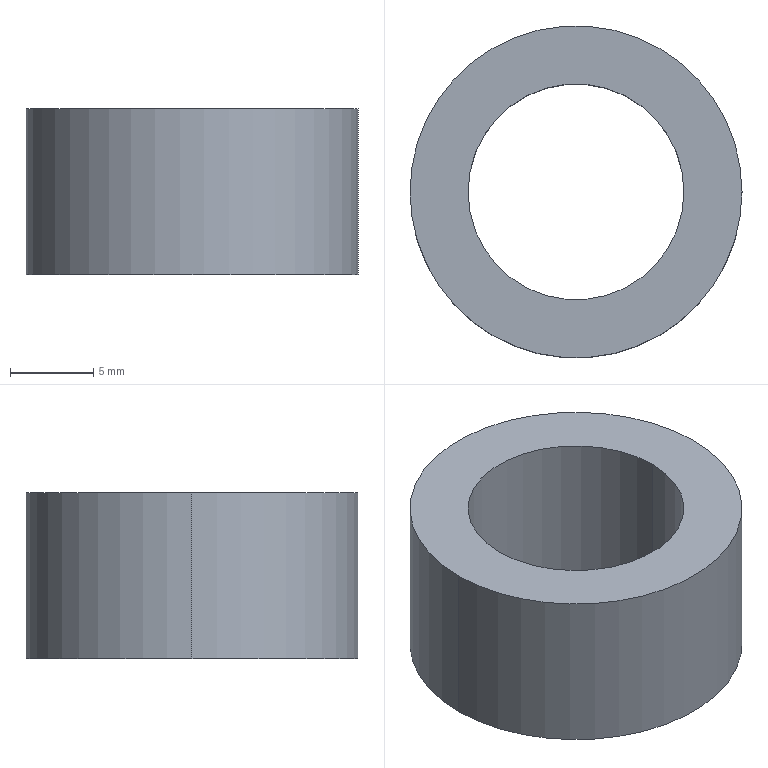Part | SolidWorks | features Cut 1, Extrusion 1 | 1 solid | 6 faces | box 20 x 20 x 10 mm | volume 1814 mm3 | cylinder 4 | plane 2 | commonest cylinder face diameters 13 x2 20 x2
STEP:
#1=CARTESIAN_POINT('',(-6.5,0.,0.));
#2=VERTEX_POINT('',#1);
#3=CARTESIAN_POINT('',(6.5,0.,0.));
#4=VERTEX_POINT('',#3);
#5=CARTESIAN_POINT('',(0.,0.,0.));
#6=DIRECTION('',(0.,0.,1.));
#7=DIRECTION('',(1.,0.,0.));
#8=AXIS2_PLACEMENT_3D('',#5,#6,#7);
#9=CIRCLE('',#8,6.5);
#10=EDGE_CURVE('',#2,#4,#9,.T.);
#11=ORIENTED_EDGE('',*,*,#10,.F.);
#12=CARTESIAN_POINT('',(-6.5,0.,10.));
#13=VERTEX_POINT('',#12);
#14=CARTESIAN_POINT('',(-6.5,0.,0.));
#15=DIRECTION('',(0.,0.,1.));
#16=VECTOR('',#15,1000.);
#17=LINE('',#14,#16);
#18=EDGE_CURVE('',#2,#13,#17,.T.);
#19=ORIENTED_EDGE('',*,*,#18,.T.);
#20=CARTESIAN_POINT('',(6.5,0.,10.));
#21=VERTEX_POINT('',#20);
#22=CARTESIAN_POINT('',(0.,0.,10.));
#23=DIRECTION('',(0.,0.,1.));
#24=DIRECTION('',(1.,0.,0.));
#25=AXIS2_PLACEMENT_3D('',#22,#23,#24);
#26=CIRCLE('',#25,6.5);
#27=EDGE_CURVE('',#13,#21,#26,.T.);
#28=ORIENTED_EDGE('',*,*,#27,.T.);
#29=CARTESIAN_POINT('',(6.5,0.,0.));
#30=DIRECTION('',(0.,0.,1.));
#31=VECTOR('',#30,1000.);
#32=LINE('',#29,#31);
#33=EDGE_CURVE('',#4,#21,#32,.T.);
#34=ORIENTED_EDGE('',*,*,#33,.F.);
#35=EDGE_LOOP('',(#11,#19,#28,#34));
#36=FACE_OUTER_BOUND('',#35,.T.);
#37=CARTESIAN_POINT('',(0.,0.,0.));
#38=DIRECTION('',(0.,0.,1.));
#39=DIRECTION('',(1.,0.,0.));
#40=AXIS2_PLACEMENT_3D('',#37,#38,#39);
#41=CYLINDRICAL_SURFACE('',#40,6.5);
#42=ADVANCED_FACE('',(#36),#41,.F.);
#43=CARTESIAN_POINT('',(10.,0.,10.));
#44=VERTEX_POINT('',#43);
#45=CARTESIAN_POINT('',(-10.,0.,10.));
#46=VERTEX_POINT('',#45);
#47=CARTESIAN_POINT('',(0.,0.,10.));
#48=DIRECTION('',(0.,0.,1.));
#49=DIRECTION('',(1.,0.,0.));
#50=AXIS2_PLACEMENT_3D('',#47,#48,#49);
#51=CIRCLE('',#50,10.);
#52=EDGE_CURVE('',#44,#46,#51,.T.);
#53=ORIENTED_EDGE('',*,*,#52,.F.);
#54=CARTESIAN_POINT('',(10.,0.,0.));
#55=VERTEX_POINT('',#54);
#56=CARTESIAN_POINT('',(10.,0.,10.));
#57=DIRECTION('',(0.,0.,-1.));
#58=VECTOR('',#57,1000.);
#59=LINE('',#56,#58);
#60=EDGE_CURVE('',#44,#55,#59,.T.);
#61=ORIENTED_EDGE('',*,*,#60,.T.);
#62=CARTESIAN_POINT('',(-10.,0.,0.));
#63=VERTEX_POINT('',#62);
#64=CARTESIAN_POINT('',(0.,0.,0.));
#65=DIRECTION('',(0.,0.,1.));
#66=DIRECTION('',(1.,0.,0.));
#67=AXIS2_PLACEMENT_3D('',#64,#65,#66);
#68=CIRCLE('',#67,10.);
#69=EDGE_CURVE('',#55,#63,#68,.T.);
#70=ORIENTED_EDGE('',*,*,#69,.T.);
#71=CARTESIAN_POINT('',(-10.,0.,10.));
#72=DIRECTION('',(0.,0.,-1.));
#73=VECTOR('',#72,1000.);
#74=LINE('',#71,#73);
#75=EDGE_CURVE('',#46,#63,#74,.T.);
#76=ORIENTED_EDGE('',*,*,#75,.F.);
#77=EDGE_LOOP('',(#53,#61,#70,#76));
#78=FACE_OUTER_BOUND('',#77,.T.);
#79=CARTESIAN_POINT('',(0.,0.,10.));
#80=DIRECTION('',(0.,0.,-1.));
#81=DIRECTION('',(-1.,0.,0.));
#82=AXIS2_PLACEMENT_3D('',#79,#80,#81);
#83=CYLINDRICAL_SURFACE('',#82,10.);
#84=ADVANCED_FACE('',(#78),#83,.T.);
#85=ORIENTED_EDGE('',*,*,#60,.F.);
#86=CARTESIAN_POINT('',(0.,0.,10.));
#87=DIRECTION('',(0.,0.,1.));
#88=DIRECTION('',(1.,0.,0.));
#89=AXIS2_PLACEMENT_3D('',#86,#87,#88);
#90=CIRCLE('',#89,10.);
#91=EDGE_CURVE('',#46,#44,#90,.T.);
#92=ORIENTED_EDGE('',*,*,#91,.F.);
#93=ORIENTED_EDGE('',*,*,#75,.T.);
#94=CARTESIAN_POINT('',(0.,0.,0.));
#95=DIRECTION('',(0.,0.,1.));
#96=DIRECTION('',(1.,0.,0.));
#97=AXIS2_PLACEMENT_3D('',#94,#95,#96);
#98=CIRCLE('',#97,10.);
#99=EDGE_CURVE('',#63,#55,#98,.T.);
#100=ORIENTED_EDGE('',*,*,#99,.T.);
#101=EDGE_LOOP('',(#85,#92,#93,#100));
#102=FACE_OUTER_BOUND('',#101,.T.);
#103=CARTESIAN_POINT('',(0.,0.,10.));
#104=DIRECTION('',(0.,0.,-1.));
#105=DIRECTION('',(-1.,0.,0.));
#106=AXIS2_PLACEMENT_3D('',#103,#104,#105);
#107=CYLINDRICAL_SURFACE('',#106,10.);
#108=ADVANCED_FACE('',(#102),#107,.T.);
#109=CARTESIAN_POINT('',(0.,0.,10.));
#110=DIRECTION('',(0.,0.,1.));
#111=DIRECTION('',(1.,0.,0.));
#112=AXIS2_PLACEMENT_3D('',#109,#110,#111);
#113=CIRCLE('',#112,6.5);
#114=EDGE_CURVE('',#21,#13,#113,.T.);
#115=ORIENTED_EDGE('',*,*,#114,.F.);
#116=ORIENTED_EDGE('',*,*,#27,.F.);
#117=EDGE_LOOP('',(#115,#116));
#118=FACE_BOUND('',#117,.T.);
#119=ORIENTED_EDGE('',*,*,#91,.T.);
#120=ORIENTED_EDGE('',*,*,#52,.T.);
#121=EDGE_LOOP('',(#119,#120));
#122=FACE_OUTER_BOUND('',#121,.T.);
#123=CARTESIAN_POINT('',(0.,0.,10.));
#124=DIRECTION('',(0.,0.,1.));
#125=DIRECTION('',(1.,0.,0.));
#126=AXIS2_PLACEMENT_3D('',#123,#124,#125);
#127=PLANE('',#126);
#128=ADVANCED_FACE('',(#118,#122),#127,.T.);
#129=CARTESIAN_POINT('',(0.,0.,0.));
#130=DIRECTION('',(0.,0.,1.));
#131=DIRECTION('',(1.,0.,0.));
#132=AXIS2_PLACEMENT_3D('',#129,#130,#131);
#133=CIRCLE('',#132,6.5);
#134=EDGE_CURVE('',#4,#2,#133,.T.);
#135=ORIENTED_EDGE('',*,*,#134,.T.);
#136=ORIENTED_EDGE('',*,*,#10,.T.);
#137=EDGE_LOOP('',(#135,#136));
#138=FACE_BOUND('',#137,.T.);
#139=ORIENTED_EDGE('',*,*,#99,.F.);
#140=ORIENTED_EDGE('',*,*,#69,.F.);
#141=EDGE_LOOP('',(#139,#140));
#142=FACE_OUTER_BOUND('',#141,.T.);
#143=CARTESIAN_POINT('',(0.,0.,0.));
#144=DIRECTION('',(0.,0.,1.));
#145=DIRECTION('',(1.,0.,0.));
#146=AXIS2_PLACEMENT_3D('',#143,#144,#145);
#147=PLANE('',#146);
#148=ADVANCED_FACE('',(#138,#142),#147,.F.);
#149=ORIENTED_EDGE('',*,*,#18,.F.);
#150=ORIENTED_EDGE('',*,*,#134,.F.);
#151=ORIENTED_EDGE('',*,*,#33,.T.);
#152=ORIENTED_EDGE('',*,*,#114,.T.);
#153=EDGE_LOOP('',(#149,#150,#151,#152));
#154=FACE_OUTER_BOUND('',#153,.T.);
#155=CARTESIAN_POINT('',(0.,0.,0.));
#156=DIRECTION('',(0.,0.,1.));
#157=DIRECTION('',(1.,0.,0.));
#158=AXIS2_PLACEMENT_3D('',#155,#156,#157);
#159=CYLINDRICAL_SURFACE('',#158,6.5);
#160=ADVANCED_FACE('',(#154),#159,.F.);
#161=CLOSED_SHELL('',(#42,#84,#108,#128,#148,#160));
#162=MANIFOLD_SOLID_BREP('',#161);
#163=CARTESIAN_POINT('',(0.,0.,0.));
#164=DIRECTION('',(0.,0.,1.));
#165=DIRECTION('',(1.,0.,0.));
#166=AXIS2_PLACEMENT_3D('',#163,#164,#165);
#167=(LENGTH_UNIT()NAMED_UNIT(*)SI_UNIT(.MILLI.,.METRE.));
#168=UNCERTAINTY_MEASURE_WITH_UNIT(LENGTH_MEASURE(0.00001),#167,'','');
#169=(NAMED_UNIT(*)PLANE_ANGLE_UNIT()SI_UNIT($,.RADIAN.));
#170=(NAMED_UNIT(*)SI_UNIT($,.STERADIAN.)SOLID_ANGLE_UNIT());
#171=(GEOMETRIC_REPRESENTATION_CONTEXT(3)GLOBAL_UNCERTAINTY_ASSIGNED_CONTEXT((#168))GLOBAL_UNIT_ASSIGNED_CONTEXT((#167,#169,#170))REPRESENTATION_CONTEXT('',''));
#172=ADVANCED_BREP_SHAPE_REPRESENTATION('',(#162,#166),#171);